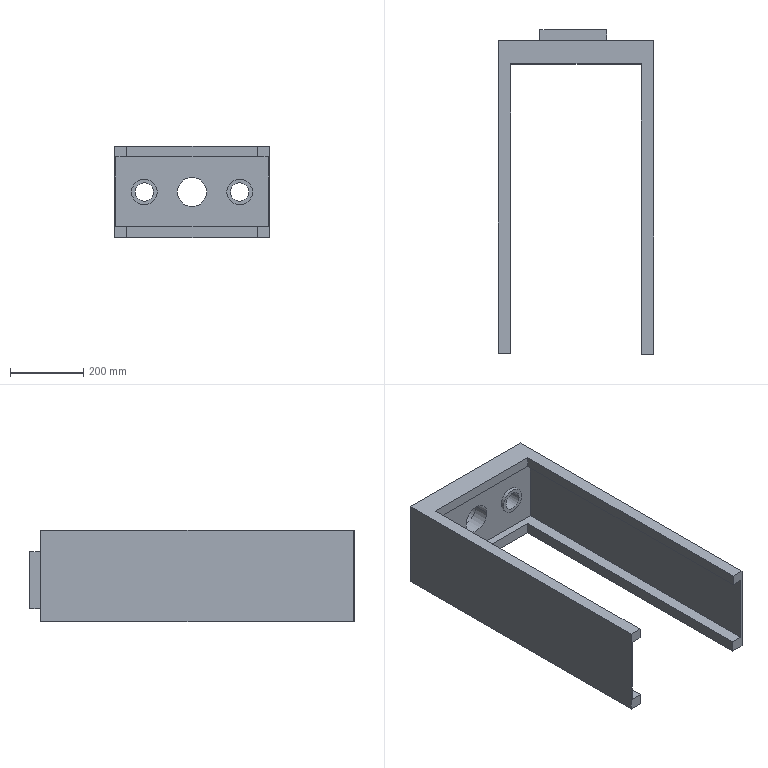Part | STEP file | Input 2 | 1 solid | 46 faces | box 425 x 886.727 x 250 mm | volume 9528731 mm3 | plane 32 | cylinder 14 | commonest cylinder face diameters 50 x4 70 x4 80 x2 85 x2 86 x2
STEP:
#1=CARTESIAN_POINT('',(-706.359,1977.264,3172.342));
#2=VERTEX_POINT('',#1);
#3=CARTESIAN_POINT('',(-791.359,1977.264,3172.342));
#4=VERTEX_POINT('',#3);
#5=CARTESIAN_POINT('',(-748.859,1977.264,3172.342));
#6=DIRECTION('',(0.,1.,0.));
#7=DIRECTION('',(1.,0.,0.));
#8=AXIS2_PLACEMENT_3D('',#5,#6,#7);
#9=CIRCLE('',#8,42.5);
#10=EDGE_CURVE('',#2,#4,#9,.T.);
#11=ORIENTED_EDGE('',*,*,#10,.F.);
#12=CARTESIAN_POINT('',(-706.359,1949.264,3172.342));
#13=VERTEX_POINT('',#12);
#14=CARTESIAN_POINT('',(-706.359,2599.264,3172.342));
#15=DIRECTION('',(0.,1.,0.));
#16=VECTOR('',#15,1000.);
#17=LINE('',#14,#16);
#18=EDGE_CURVE('',#13,#2,#17,.T.);
#19=ORIENTED_EDGE('',*,*,#18,.F.);
#20=CARTESIAN_POINT('',(-791.359,1949.264,3172.342));
#21=VERTEX_POINT('',#20);
#22=CARTESIAN_POINT('',(-748.859,1949.264,3172.342));
#23=DIRECTION('',(0.,1.,0.));
#24=DIRECTION('',(-1.,0.,0.));
#25=AXIS2_PLACEMENT_3D('',#22,#23,#24);
#26=CIRCLE('',#25,42.5);
#27=EDGE_CURVE('',#13,#21,#26,.T.);
#28=ORIENTED_EDGE('',*,*,#27,.T.);
#29=CARTESIAN_POINT('',(-791.359,2599.264,3172.342));
#30=DIRECTION('',(0.,1.,0.));
#31=VECTOR('',#30,1000.);
#32=LINE('',#29,#31);
#33=EDGE_CURVE('',#21,#4,#32,.T.);
#34=ORIENTED_EDGE('',*,*,#33,.T.);
#35=EDGE_LOOP('',(#11,#19,#28,#34));
#36=FACE_OUTER_BOUND('',#35,.T.);
#37=CARTESIAN_POINT('',(-748.859,2599.264,3172.342));
#38=DIRECTION('',(0.,-1.,0.));
#39=DIRECTION('',(1.,0.,0.));
#40=AXIS2_PLACEMENT_3D('',#37,#38,#39);
#41=CYLINDRICAL_SURFACE('',#40,42.5);
#42=ADVANCED_FACE('',(#36),#41,.T.);
#43=CARTESIAN_POINT('',(-791.859,1977.264,3172.342));
#44=VERTEX_POINT('',#43);
#45=CARTESIAN_POINT('',(-705.859,1977.264,3172.342));
#46=VERTEX_POINT('',#45);
#47=CARTESIAN_POINT('',(-748.859,1977.264,3172.342));
#48=DIRECTION('',(0.,1.,0.));
#49=DIRECTION('',(1.,0.,0.));
#50=AXIS2_PLACEMENT_3D('',#47,#48,#49);
#51=CIRCLE('',#50,43.);
#52=EDGE_CURVE('',#44,#46,#51,.T.);
#53=ORIENTED_EDGE('',*,*,#52,.F.);
#54=CARTESIAN_POINT('',(-791.859,1979.264,3172.342));
#55=VERTEX_POINT('',#54);
#56=CARTESIAN_POINT('',(-791.859,1977.264,3172.342));
#57=DIRECTION('',(0.,1.,0.));
#58=VECTOR('',#57,1000.);
#59=LINE('',#56,#58);
#60=EDGE_CURVE('',#44,#55,#59,.T.);
#61=ORIENTED_EDGE('',*,*,#60,.T.);
#62=CARTESIAN_POINT('',(-705.859,1979.264,3172.342));
#63=VERTEX_POINT('',#62);
#64=CARTESIAN_POINT('',(-748.859,1979.264,3172.342));
#65=DIRECTION('',(0.,1.,0.));
#66=DIRECTION('',(1.,0.,0.));
#67=AXIS2_PLACEMENT_3D('',#64,#65,#66);
#68=CIRCLE('',#67,43.);
#69=EDGE_CURVE('',#55,#63,#68,.T.);
#70=ORIENTED_EDGE('',*,*,#69,.T.);
#71=CARTESIAN_POINT('',(-705.859,1977.264,3172.342));
#72=DIRECTION('',(0.,1.,0.));
#73=VECTOR('',#72,1000.);
#74=LINE('',#71,#73);
#75=EDGE_CURVE('',#46,#63,#74,.T.);
#76=ORIENTED_EDGE('',*,*,#75,.F.);
#77=EDGE_LOOP('',(#53,#61,#70,#76));
#78=FACE_OUTER_BOUND('',#77,.T.);
#79=CARTESIAN_POINT('',(-748.859,1977.264,3172.342));
#80=DIRECTION('',(0.,1.,0.));
#81=DIRECTION('',(-1.,0.,0.));
#82=AXIS2_PLACEMENT_3D('',#79,#80,#81);
#83=CYLINDRICAL_SURFACE('',#82,43.);
#84=ADVANCED_FACE('',(#78),#83,.F.);
#85=CARTESIAN_POINT('',(-653.859,1895.264,3172.342));
#86=VERTEX_POINT('',#85);
#87=CARTESIAN_POINT('',(-583.859,1895.264,3172.342));
#88=VERTEX_POINT('',#87);
#89=CARTESIAN_POINT('',(-618.859,1895.264,3172.342));
#90=DIRECTION('',(0.,-1.,0.));
#91=DIRECTION('',(1.,0.,0.));
#92=AXIS2_PLACEMENT_3D('',#89,#90,#91);
#93=CIRCLE('',#92,35.);
#94=EDGE_CURVE('',#86,#88,#93,.T.);
#95=ORIENTED_EDGE('',*,*,#94,.F.);
#96=CARTESIAN_POINT('',(-653.859,1905.264,3172.342));
#97=VERTEX_POINT('',#96);
#98=CARTESIAN_POINT('',(-653.859,1895.264,3172.342));
#99=DIRECTION('',(0.,1.,0.));
#100=VECTOR('',#99,1000.);
#101=LINE('',#98,#100);
#102=EDGE_CURVE('',#86,#97,#101,.T.);
#103=ORIENTED_EDGE('',*,*,#102,.T.);
#104=CARTESIAN_POINT('',(-583.859,1905.264,3172.342));
#105=VERTEX_POINT('',#104);
#106=CARTESIAN_POINT('',(-618.859,1905.264,3172.342));
#107=DIRECTION('',(0.,-1.,0.));
#108=DIRECTION('',(1.,0.,0.));
#109=AXIS2_PLACEMENT_3D('',#106,#107,#108);
#110=CIRCLE('',#109,35.);
#111=EDGE_CURVE('',#97,#105,#110,.T.);
#112=ORIENTED_EDGE('',*,*,#111,.T.);
#113=CARTESIAN_POINT('',(-583.859,1895.264,3172.342));
#114=DIRECTION('',(0.,1.,0.));
#115=VECTOR('',#114,1000.);
#116=LINE('',#113,#115);
#117=EDGE_CURVE('',#88,#105,#116,.T.);
#118=ORIENTED_EDGE('',*,*,#117,.F.);
#119=EDGE_LOOP('',(#95,#103,#112,#118));
#120=FACE_OUTER_BOUND('',#119,.T.);
#121=CARTESIAN_POINT('',(-618.859,1895.264,3172.342));
#122=DIRECTION('',(0.,1.,0.));
#123=DIRECTION('',(-1.,0.,0.));
#124=AXIS2_PLACEMENT_3D('',#121,#122,#123);
#125=CYLINDRICAL_SURFACE('',#124,35.);
#126=ADVANCED_FACE('',(#120),#125,.T.);
#127=CARTESIAN_POINT('',(-913.859,1895.264,3172.342));
#128=VERTEX_POINT('',#127);
#129=CARTESIAN_POINT('',(-843.859,1895.264,3172.342));
#130=VERTEX_POINT('',#129);
#131=CARTESIAN_POINT('',(-878.859,1895.264,3172.342));
#132=DIRECTION('',(0.,-1.,0.));
#133=DIRECTION('',(-1.,0.,0.));
#134=AXIS2_PLACEMENT_3D('',#131,#132,#133);
#135=CIRCLE('',#134,35.);
#136=EDGE_CURVE('',#128,#130,#135,.T.);
#137=ORIENTED_EDGE('',*,*,#136,.F.);
#138=CARTESIAN_POINT('',(-913.859,1905.264,3172.342));
#139=VERTEX_POINT('',#138);
#140=CARTESIAN_POINT('',(-913.859,1895.264,3172.342));
#141=DIRECTION('',(0.,1.,0.));
#142=VECTOR('',#141,1000.);
#143=LINE('',#140,#142);
#144=EDGE_CURVE('',#128,#139,#143,.T.);
#145=ORIENTED_EDGE('',*,*,#144,.T.);
#146=CARTESIAN_POINT('',(-843.859,1905.264,3172.342));
#147=VERTEX_POINT('',#146);
#148=CARTESIAN_POINT('',(-878.859,1905.264,3172.342));
#149=DIRECTION('',(0.,-1.,0.));
#150=DIRECTION('',(1.,0.,0.));
#151=AXIS2_PLACEMENT_3D('',#148,#149,#150);
#152=CIRCLE('',#151,35.);
#153=EDGE_CURVE('',#139,#147,#152,.T.);
#154=ORIENTED_EDGE('',*,*,#153,.T.);
#155=CARTESIAN_POINT('',(-843.859,1895.264,3172.342));
#156=DIRECTION('',(0.,1.,0.));
#157=VECTOR('',#156,1000.);
#158=LINE('',#155,#157);
#159=EDGE_CURVE('',#130,#147,#158,.T.);
#160=ORIENTED_EDGE('',*,*,#159,.F.);
#161=EDGE_LOOP('',(#137,#145,#154,#160));
#162=FACE_OUTER_BOUND('',#161,.T.);
#163=CARTESIAN_POINT('',(-878.859,1895.264,3172.342));
#164=DIRECTION('',(0.,1.,0.));
#165=DIRECTION('',(-1.,0.,0.));
#166=AXIS2_PLACEMENT_3D('',#163,#164,#165);
#167=CYLINDRICAL_SURFACE('',#166,35.);
#168=ADVANCED_FACE('',(#162),#167,.T.);
#169=CARTESIAN_POINT('',(-853.859,1949.264,3172.342));
#170=VERTEX_POINT('',#169);
#171=CARTESIAN_POINT('',(-903.859,1949.264,3172.342));
#172=VERTEX_POINT('',#171);
#173=CARTESIAN_POINT('',(-878.859,1949.264,3172.342));
#174=DIRECTION('',(0.,-1.,0.));
#175=DIRECTION('',(-1.,0.,0.));
#176=AXIS2_PLACEMENT_3D('',#173,#174,#175);
#177=CIRCLE('',#176,25.);
#178=EDGE_CURVE('',#170,#172,#177,.T.);
#179=ORIENTED_EDGE('',*,*,#178,.F.);
#180=CARTESIAN_POINT('',(-853.859,1895.264,3172.342));
#181=VERTEX_POINT('',#180);
#182=CARTESIAN_POINT('',(-853.859,2789.264,3172.342));
#183=DIRECTION('',(0.,1.,0.));
#184=VECTOR('',#183,1000.);
#185=LINE('',#182,#184);
#186=EDGE_CURVE('',#181,#170,#185,.T.);
#187=ORIENTED_EDGE('',*,*,#186,.F.);
#188=CARTESIAN_POINT('',(-903.859,1895.264,3172.342));
#189=VERTEX_POINT('',#188);
#190=CARTESIAN_POINT('',(-878.859,1895.264,3172.342));
#191=DIRECTION('',(0.,-1.,0.));
#192=DIRECTION('',(-1.,0.,0.));
#193=AXIS2_PLACEMENT_3D('',#190,#191,#192);
#194=CIRCLE('',#193,25.);
#195=EDGE_CURVE('',#181,#189,#194,.T.);
#196=ORIENTED_EDGE('',*,*,#195,.T.);
#197=CARTESIAN_POINT('',(-903.859,2789.264,3172.342));
#198=DIRECTION('',(0.,1.,0.));
#199=VECTOR('',#198,1000.);
#200=LINE('',#197,#199);
#201=EDGE_CURVE('',#189,#172,#200,.T.);
#202=ORIENTED_EDGE('',*,*,#201,.T.);
#203=EDGE_LOOP('',(#179,#187,#196,#202));
#204=FACE_OUTER_BOUND('',#203,.T.);
#205=CARTESIAN_POINT('',(-878.859,2789.264,3172.342));
#206=DIRECTION('',(0.,-1.,0.));
#207=DIRECTION('',(1.,0.,0.));
#208=AXIS2_PLACEMENT_3D('',#205,#206,#207);
#209=CYLINDRICAL_SURFACE('',#208,25.);
#210=ADVANCED_FACE('',(#204),#209,.F.);
#211=CARTESIAN_POINT('',(-593.859,1949.264,3172.342));
#212=VERTEX_POINT('',#211);
#213=CARTESIAN_POINT('',(-643.859,1949.264,3172.342));
#214=VERTEX_POINT('',#213);
#215=CARTESIAN_POINT('',(-618.859,1949.264,3172.342));
#216=DIRECTION('',(0.,-1.,0.));
#217=DIRECTION('',(-1.,0.,0.));
#218=AXIS2_PLACEMENT_3D('',#215,#216,#217);
#219=CIRCLE('',#218,25.);
#220=EDGE_CURVE('',#212,#214,#219,.T.);
#221=ORIENTED_EDGE('',*,*,#220,.F.);
#222=CARTESIAN_POINT('',(-593.859,1895.264,3172.342));
#223=VERTEX_POINT('',#222);
#224=CARTESIAN_POINT('',(-593.859,2789.264,3172.342));
#225=DIRECTION('',(0.,1.,0.));
#226=VECTOR('',#225,1000.);
#227=LINE('',#224,#226);
#228=EDGE_CURVE('',#223,#212,#227,.T.);
#229=ORIENTED_EDGE('',*,*,#228,.F.);
#230=CARTESIAN_POINT('',(-643.859,1895.264,3172.342));
#231=VERTEX_POINT('',#230);
#232=CARTESIAN_POINT('',(-618.859,1895.264,3172.342));
#233=DIRECTION('',(0.,-1.,0.));
#234=DIRECTION('',(-1.,0.,0.));
#235=AXIS2_PLACEMENT_3D('',#232,#233,#234);
#236=CIRCLE('',#235,25.);
#237=EDGE_CURVE('',#223,#231,#236,.T.);
#238=ORIENTED_EDGE('',*,*,#237,.T.);
#239=CARTESIAN_POINT('',(-643.859,2789.264,3172.342));
#240=DIRECTION('',(0.,1.,0.));
#241=VECTOR('',#240,1000.);
#242=LINE('',#239,#241);
#243=EDGE_CURVE('',#231,#214,#242,.T.);
#244=ORIENTED_EDGE('',*,*,#243,.T.);
#245=EDGE_LOOP('',(#221,#229,#238,#244));
#246=FACE_OUTER_BOUND('',#245,.T.);
#247=CARTESIAN_POINT('',(-618.859,2789.264,3172.342));
#248=DIRECTION('',(0.,-1.,0.));
#249=DIRECTION('',(1.,0.,0.));
#250=AXIS2_PLACEMENT_3D('',#247,#248,#249);
#251=CYLINDRICAL_SURFACE('',#250,25.);
#252=ADVANCED_FACE('',(#246),#251,.F.);
#253=CARTESIAN_POINT('',(-708.859,1977.264,3172.342));
#254=VERTEX_POINT('',#253);
#255=CARTESIAN_POINT('',(-788.859,1977.264,3172.342));
#256=VERTEX_POINT('',#255);
#257=CARTESIAN_POINT('',(-748.859,1977.264,3172.342));
#258=DIRECTION('',(0.,-1.,0.));
#259=DIRECTION('',(1.,0.,0.));
#260=AXIS2_PLACEMENT_3D('',#257,#258,#259);
#261=CIRCLE('',#260,40.);
#262=EDGE_CURVE('',#254,#256,#261,.T.);
#263=ORIENTED_EDGE('',*,*,#262,.F.);
#264=CARTESIAN_POINT('',(-708.859,1905.264,3172.342));
#265=VERTEX_POINT('',#264);
#266=CARTESIAN_POINT('',(-708.859,2829.064,3172.342));
#267=DIRECTION('',(0.,1.,0.));
#268=VECTOR('',#267,1000.);
#269=LINE('',#266,#268);
#270=EDGE_CURVE('',#265,#254,#269,.T.);
#271=ORIENTED_EDGE('',*,*,#270,.F.);
#272=CARTESIAN_POINT('',(-788.859,1905.264,3172.342));
#273=VERTEX_POINT('',#272);
#274=CARTESIAN_POINT('',(-748.859,1905.264,3172.342));
#275=DIRECTION('',(0.,1.,0.));
#276=DIRECTION('',(1.,0.,0.));
#277=AXIS2_PLACEMENT_3D('',#274,#275,#276);
#278=CIRCLE('',#277,40.);
#279=EDGE_CURVE('',#273,#265,#278,.T.);
#280=ORIENTED_EDGE('',*,*,#279,.F.);
#281=CARTESIAN_POINT('',(-788.859,2829.064,3172.342));
#282=DIRECTION('',(0.,1.,0.));
#283=VECTOR('',#282,1000.);
#284=LINE('',#281,#283);
#285=EDGE_CURVE('',#273,#256,#284,.T.);
#286=ORIENTED_EDGE('',*,*,#285,.T.);
#287=EDGE_LOOP('',(#263,#271,#280,#286));
#288=FACE_OUTER_BOUND('',#287,.T.);
#289=CARTESIAN_POINT('',(-748.859,2829.064,3172.342));
#290=DIRECTION('',(0.,-1.,0.));
#291=DIRECTION('',(1.,0.,0.));
#292=AXIS2_PLACEMENT_3D('',#289,#290,#291);
#293=CYLINDRICAL_SURFACE('',#292,40.);
#294=ADVANCED_FACE('',(#288),#293,.F.);
#295=CARTESIAN_POINT('',(-961.359,1949.264,3047.342));
#296=VERTEX_POINT('',#295);
#297=CARTESIAN_POINT('',(-961.359,1095.094,3047.342));
#298=VERTEX_POINT('',#297);
#299=CARTESIAN_POINT('',(-961.359,1949.264,3047.342));
#300=DIRECTION('',(0.,-1.,0.));
#301=VECTOR('',#300,1000.);
#302=LINE('',#299,#301);
#303=EDGE_CURVE('',#296,#298,#302,.T.);
#304=ORIENTED_EDGE('',*,*,#303,.T.);
#305=CARTESIAN_POINT('',(-961.359,1095.094,3297.342));
#306=VERTEX_POINT('',#305);
#307=CARTESIAN_POINT('',(-961.359,1095.094,4799.342));
#308=DIRECTION('',(0.,0.,-1.));
#309=VECTOR('',#308,1000.);
#310=LINE('',#307,#309);
#311=EDGE_CURVE('',#306,#298,#310,.T.);
#312=ORIENTED_EDGE('',*,*,#311,.F.);
#313=CARTESIAN_POINT('',(-961.359,1949.264,3297.342));
#314=VERTEX_POINT('',#313);
#315=CARTESIAN_POINT('',(-961.359,1949.264,3297.342));
#316=DIRECTION('',(0.,-1.,0.));
#317=VECTOR('',#316,1000.);
#318=LINE('',#315,#317);
#319=EDGE_CURVE('',#314,#306,#318,.T.);
#320=ORIENTED_EDGE('',*,*,#319,.F.);
#321=CARTESIAN_POINT('',(-961.359,1949.264,3297.342));
#322=DIRECTION('',(0.,0.,1.));
#323=VECTOR('',#322,1000.);
#324=LINE('',#321,#323);
#325=EDGE_CURVE('',#296,#314,#324,.T.);
#326=ORIENTED_EDGE('',*,*,#325,.F.);
#327=EDGE_LOOP('',(#304,#312,#320,#326));
#328=FACE_OUTER_BOUND('',#327,.T.);
#329=CARTESIAN_POINT('',(-961.359,1949.264,3297.342));
#330=DIRECTION('',(1.,0.,0.));
#331=DIRECTION('',(0.,1.,0.));
#332=AXIS2_PLACEMENT_3D('',#329,#330,#331);
#333=PLANE('',#332);
#334=ADVANCED_FACE('',(#328),#333,.F.);
#335=CARTESIAN_POINT('',(-536.359,1949.264,3297.342));
#336=VERTEX_POINT('',#335);
#337=CARTESIAN_POINT('',(-536.359,1092.538,3297.342));
#338=VERTEX_POINT('',#337);
#339=CARTESIAN_POINT('',(-536.359,1949.264,3297.342));
#340=DIRECTION('',(0.,-1.,0.));
#341=VECTOR('',#340,1000.);
#342=LINE('',#339,#341);
#343=EDGE_CURVE('',#336,#338,#342,.T.);
#344=ORIENTED_EDGE('',*,*,#343,.T.);
#345=CARTESIAN_POINT('',(-536.359,1092.538,3047.342));
#346=VERTEX_POINT('',#345);
#347=CARTESIAN_POINT('',(-536.359,1092.538,4799.342));
#348=DIRECTION('',(0.,0.,-1.));
#349=VECTOR('',#348,1000.);
#350=LINE('',#347,#349);
#351=EDGE_CURVE('',#338,#346,#350,.T.);
#352=ORIENTED_EDGE('',*,*,#351,.T.);
#353=CARTESIAN_POINT('',(-536.359,1949.264,3047.342));
#354=VERTEX_POINT('',#353);
#355=CARTESIAN_POINT('',(-536.359,1949.264,3047.342));
#356=DIRECTION('',(0.,-1.,0.));
#357=VECTOR('',#356,1000.);
#358=LINE('',#355,#357);
#359=EDGE_CURVE('',#354,#346,#358,.T.);
#360=ORIENTED_EDGE('',*,*,#359,.F.);
#361=CARTESIAN_POINT('',(-536.359,1949.264,3297.342));
#362=DIRECTION('',(0.,0.,-1.));
#363=VECTOR('',#362,1000.);
#364=LINE('',#361,#363);
#365=EDGE_CURVE('',#336,#354,#364,.T.);
#366=ORIENTED_EDGE('',*,*,#365,.F.);
#367=EDGE_LOOP('',(#344,#352,#360,#366));
#368=FACE_OUTER_BOUND('',#367,.T.);
#369=CARTESIAN_POINT('',(-536.359,1949.264,3297.342));
#370=DIRECTION('',(-1.,0.,0.));
#371=DIRECTION('',(0.,-1.,0.));
#372=AXIS2_PLACEMENT_3D('',#369,#370,#371);
#373=PLANE('',#372);
#374=ADVANCED_FACE('',(#368),#373,.F.);
#375=ORIENTED_EDGE('',*,*,#359,.T.);
#376=CARTESIAN_POINT('',(-571.359,1092.538,3047.342));
#377=VERTEX_POINT('',#376);
#378=CARTESIAN_POINT('',(-683.964,1092.538,3047.342));
#379=DIRECTION('',(1.,0.,0.));
#380=VECTOR('',#379,1000.);
#381=LINE('',#378,#380);
#382=EDGE_CURVE('',#377,#346,#381,.T.);
#383=ORIENTED_EDGE('',*,*,#382,.F.);
#384=CARTESIAN_POINT('',(-571.359,1884.264,3047.342));
#385=VERTEX_POINT('',#384);
#386=CARTESIAN_POINT('',(-571.359,890.264,3047.342));
#387=DIRECTION('',(0.,-1.,0.));
#388=VECTOR('',#387,1000.);
#389=LINE('',#386,#388);
#390=EDGE_CURVE('',#385,#377,#389,.T.);
#391=ORIENTED_EDGE('',*,*,#390,.F.);
#392=CARTESIAN_POINT('',(-926.359,1884.264,3047.342));
#393=VERTEX_POINT('',#392);
#394=CARTESIAN_POINT('',(-926.359,1884.264,3047.342));
#395=DIRECTION('',(1.,0.,0.));
#396=VECTOR('',#395,1000.);
#397=LINE('',#394,#396);
#398=EDGE_CURVE('',#393,#385,#397,.T.);
#399=ORIENTED_EDGE('',*,*,#398,.F.);
#400=CARTESIAN_POINT('',(-926.359,1095.094,3047.342));
#401=VERTEX_POINT('',#400);
#402=CARTESIAN_POINT('',(-926.359,890.264,3047.342));
#403=DIRECTION('',(0.,1.,0.));
#404=VECTOR('',#403,1000.);
#405=LINE('',#402,#404);
#406=EDGE_CURVE('',#401,#393,#405,.T.);
#407=ORIENTED_EDGE('',*,*,#406,.F.);
#408=CARTESIAN_POINT('',(-819.635,1095.094,3047.342));
#409=DIRECTION('',(1.,0.,0.));
#410=VECTOR('',#409,1000.);
#411=LINE('',#408,#410);
#412=EDGE_CURVE('',#298,#401,#411,.T.);
#413=ORIENTED_EDGE('',*,*,#412,.F.);
#414=ORIENTED_EDGE('',*,*,#303,.F.);
#415=CARTESIAN_POINT('',(-961.359,1949.264,3047.342));
#416=DIRECTION('',(-1.,0.,0.));
#417=VECTOR('',#416,1000.);
#418=LINE('',#415,#417);
#419=EDGE_CURVE('',#354,#296,#418,.T.);
#420=ORIENTED_EDGE('',*,*,#419,.F.);
#421=EDGE_LOOP('',(#375,#383,#391,#399,#407,#413,#414,#420));
#422=FACE_OUTER_BOUND('',#421,.T.);
#423=CARTESIAN_POINT('',(-961.359,1949.264,3047.342));
#424=DIRECTION('',(0.,0.,1.));
#425=DIRECTION('',(0.,1.,0.));
#426=AXIS2_PLACEMENT_3D('',#423,#424,#425);
#427=PLANE('',#426);
#428=ADVANCED_FACE('',(#422),#427,.F.);
#429=CARTESIAN_POINT('',(-570.359,1885.264,3297.342));
#430=VERTEX_POINT('',#429);
#431=CARTESIAN_POINT('',(-570.359,1092.538,3297.342));
#432=VERTEX_POINT('',#431);
#433=CARTESIAN_POINT('',(-570.359,1949.264,3297.342));
#434=DIRECTION('',(0.,-1.,0.));
#435=VECTOR('',#434,1000.);
#436=LINE('',#433,#435);
#437=EDGE_CURVE('',#430,#432,#436,.T.);
#438=ORIENTED_EDGE('',*,*,#437,.T.);
#439=CARTESIAN_POINT('',(-961.359,1092.538,3297.342));
#440=DIRECTION('',(1.,0.,0.));
#441=VECTOR('',#440,1000.);
#442=LINE('',#439,#441);
#443=EDGE_CURVE('',#432,#338,#442,.T.);
#444=ORIENTED_EDGE('',*,*,#443,.T.);
#445=ORIENTED_EDGE('',*,*,#343,.F.);
#446=CARTESIAN_POINT('',(-961.359,1949.264,3297.342));
#447=DIRECTION('',(1.,0.,0.));
#448=VECTOR('',#447,1000.);
#449=LINE('',#446,#448);
#450=EDGE_CURVE('',#314,#336,#449,.T.);
#451=ORIENTED_EDGE('',*,*,#450,.F.);
#452=ORIENTED_EDGE('',*,*,#319,.T.);
#453=CARTESIAN_POINT('',(-927.359,1095.094,3297.342));
#454=VERTEX_POINT('',#453);
#455=CARTESIAN_POINT('',(-961.359,1095.094,3297.342));
#456=DIRECTION('',(1.,0.,0.));
#457=VECTOR('',#456,1000.);
#458=LINE('',#455,#457);
#459=EDGE_CURVE('',#306,#454,#458,.T.);
#460=ORIENTED_EDGE('',*,*,#459,.T.);
#461=CARTESIAN_POINT('',(-927.359,1885.264,3297.342));
#462=VERTEX_POINT('',#461);
#463=CARTESIAN_POINT('',(-927.359,1949.264,3297.342));
#464=DIRECTION('',(0.,1.,0.));
#465=VECTOR('',#464,1000.);
#466=LINE('',#463,#465);
#467=EDGE_CURVE('',#454,#462,#466,.T.);
#468=ORIENTED_EDGE('',*,*,#467,.T.);
#469=CARTESIAN_POINT('',(-961.359,1885.264,3297.342));
#470=DIRECTION('',(1.,0.,0.));
#471=VECTOR('',#470,1000.);
#472=LINE('',#469,#471);
#473=EDGE_CURVE('',#462,#430,#472,.T.);
#474=ORIENTED_EDGE('',*,*,#473,.T.);
#475=EDGE_LOOP('',(#438,#444,#445,#451,#452,#460,#468,#474));
#476=FACE_OUTER_BOUND('',#475,.T.);
#477=CARTESIAN_POINT('',(-961.359,1949.264,3297.342));
#478=DIRECTION('',(0.,0.,-1.));
#479=DIRECTION('',(0.,-1.,0.));
#480=AXIS2_PLACEMENT_3D('',#477,#478,#479);
#481=PLANE('',#480);
#482=ADVANCED_FACE('',(#476),#481,.F.);
#483=CARTESIAN_POINT('',(-571.359,1884.264,3078.342));
#484=VERTEX_POINT('',#483);
#485=CARTESIAN_POINT('',(-571.359,1092.538,3078.342));
#486=VERTEX_POINT('',#485);
#487=CARTESIAN_POINT('',(-571.359,890.264,3078.342));
#488=DIRECTION('',(0.,-1.,0.));
#489=VECTOR('',#488,1000.);
#490=LINE('',#487,#489);
#491=EDGE_CURVE('',#484,#486,#490,.T.);
#492=ORIENTED_EDGE('',*,*,#491,.T.);
#493=CARTESIAN_POINT('',(-540.359,1092.538,3078.342));
#494=VERTEX_POINT('',#493);
#495=CARTESIAN_POINT('',(-748.859,1092.538,3078.342));
#496=DIRECTION('',(1.,0.,0.));
#497=VECTOR('',#496,1000.);
#498=LINE('',#495,#497);
#499=EDGE_CURVE('',#486,#494,#498,.T.);
#500=ORIENTED_EDGE('',*,*,#499,.T.);
#501=CARTESIAN_POINT('',(-540.359,1905.264,3078.342));
#502=VERTEX_POINT('',#501);
#503=CARTESIAN_POINT('',(-540.359,869.264,3078.342));
#504=DIRECTION('',(0.,-1.,0.));
#505=VECTOR('',#504,1000.);
#506=LINE('',#503,#505);
#507=EDGE_CURVE('',#502,#494,#506,.T.);
#508=ORIENTED_EDGE('',*,*,#507,.F.);
#509=CARTESIAN_POINT('',(-957.359,1905.264,3078.342));
#510=VERTEX_POINT('',#509);
#511=CARTESIAN_POINT('',(-957.359,1905.264,3078.342));
#512=DIRECTION('',(1.,0.,0.));
#513=VECTOR('',#512,1000.);
#514=LINE('',#511,#513);
#515=EDGE_CURVE('',#510,#502,#514,.T.);
#516=ORIENTED_EDGE('',*,*,#515,.F.);
#517=CARTESIAN_POINT('',(-957.359,1095.094,3078.342));
#518=VERTEX_POINT('',#517);
#519=CARTESIAN_POINT('',(-957.359,869.264,3078.342));
#520=DIRECTION('',(0.,1.,0.));
#521=VECTOR('',#520,1000.);
#522=LINE('',#519,#521);
#523=EDGE_CURVE('',#518,#510,#522,.T.);
#524=ORIENTED_EDGE('',*,*,#523,.F.);
#525=CARTESIAN_POINT('',(-926.359,1095.094,3078.342));
#526=VERTEX_POINT('',#525);
#527=CARTESIAN_POINT('',(-748.859,1095.094,3078.342));
#528=DIRECTION('',(1.,0.,0.));
#529=VECTOR('',#528,1000.);
#530=LINE('',#527,#529);
#531=EDGE_CURVE('',#518,#526,#530,.T.);
#532=ORIENTED_EDGE('',*,*,#531,.T.);
#533=CARTESIAN_POINT('',(-926.359,1884.264,3078.342));
#534=VERTEX_POINT('',#533);
#535=CARTESIAN_POINT('',(-926.359,890.264,3078.342));
#536=DIRECTION('',(0.,1.,0.));
#537=VECTOR('',#536,1000.);
#538=LINE('',#535,#537);
#539=EDGE_CURVE('',#526,#534,#538,.T.);
#540=ORIENTED_EDGE('',*,*,#539,.T.);
#541=CARTESIAN_POINT('',(-926.359,1884.264,3078.342));
#542=DIRECTION('',(1.,0.,0.));
#543=VECTOR('',#542,1000.);
#544=LINE('',#541,#543);
#545=EDGE_CURVE('',#534,#484,#544,.T.);
#546=ORIENTED_EDGE('',*,*,#545,.T.);
#547=EDGE_LOOP('',(#492,#500,#508,#516,#524,#532,#540,#546));
#548=FACE_OUTER_BOUND('',#547,.T.);
#549=CARTESIAN_POINT('',(-748.859,825.264,3078.342));
#550=DIRECTION('',(0.,0.,-1.));
#551=DIRECTION('',(0.,-1.,0.));
#552=AXIS2_PLACEMENT_3D('',#549,#550,#551);
#553=PLANE('',#552);
#554=ADVANCED_FACE('',(#548),#553,.F.);
#555=CARTESIAN_POINT('',(-957.359,1095.094,3268.342));
#556=VERTEX_POINT('',#555);
#557=CARTESIAN_POINT('',(-957.359,1905.264,3268.342));
#558=VERTEX_POINT('',#557);
#559=CARTESIAN_POINT('',(-957.359,869.264,3268.342));
#560=DIRECTION('',(0.,1.,0.));
#561=VECTOR('',#560,1000.);
#562=LINE('',#559,#561);
#563=EDGE_CURVE('',#556,#558,#562,.T.);
#564=ORIENTED_EDGE('',*,*,#563,.F.);
#565=CARTESIAN_POINT('',(-957.359,1095.094,3268.342));
#566=DIRECTION('',(0.,0.,-1.));
#567=VECTOR('',#566,1000.);
#568=LINE('',#565,#567);
#569=EDGE_CURVE('',#556,#518,#568,.T.);
#570=ORIENTED_EDGE('',*,*,#569,.T.);
#571=ORIENTED_EDGE('',*,*,#523,.T.);
#572=CARTESIAN_POINT('',(-957.359,1905.264,3268.342));
#573=DIRECTION('',(0.,0.,-1.));
#574=VECTOR('',#573,1000.);
#575=LINE('',#572,#574);
#576=EDGE_CURVE('',#558,#510,#575,.T.);
#577=ORIENTED_EDGE('',*,*,#576,.F.);
#578=EDGE_LOOP('',(#564,#570,#571,#577));
#579=FACE_OUTER_BOUND('',#578,.T.);
#580=CARTESIAN_POINT('',(-957.359,869.264,3268.342));
#581=DIRECTION('',(-1.,0.,0.));
#582=DIRECTION('',(0.,-1.,0.));
#583=AXIS2_PLACEMENT_3D('',#580,#581,#582);
#584=PLANE('',#583);
#585=ADVANCED_FACE('',(#579),#584,.F.);
#586=ORIENTED_EDGE('',*,*,#507,.T.);
#587=CARTESIAN_POINT('',(-540.359,1092.538,3268.342));
#588=VERTEX_POINT('',#587);
#589=CARTESIAN_POINT('',(-540.359,1092.538,3268.342));
#590=DIRECTION('',(0.,0.,1.));
#591=VECTOR('',#590,1000.);
#592=LINE('',#589,#591);
#593=EDGE_CURVE('',#494,#588,#592,.T.);
#594=ORIENTED_EDGE('',*,*,#593,.T.);
#595=CARTESIAN_POINT('',(-540.359,1905.264,3268.342));
#596=VERTEX_POINT('',#595);
#597=CARTESIAN_POINT('',(-540.359,869.264,3268.342));
#598=DIRECTION('',(0.,-1.,0.));
#599=VECTOR('',#598,1000.);
#600=LINE('',#597,#599);
#601=EDGE_CURVE('',#596,#588,#600,.T.);
#602=ORIENTED_EDGE('',*,*,#601,.F.);
#603=CARTESIAN_POINT('',(-540.359,1905.264,3268.342));
#604=DIRECTION('',(0.,0.,-1.));
#605=VECTOR('',#604,1000.);
#606=LINE('',#603,#605);
#607=EDGE_CURVE('',#596,#502,#606,.T.);
#608=ORIENTED_EDGE('',*,*,#607,.T.);
#609=EDGE_LOOP('',(#586,#594,#602,#608));
#610=FACE_OUTER_BOUND('',#609,.T.);
#611=CARTESIAN_POINT('',(-540.359,869.264,3268.342));
#612=DIRECTION('',(1.,0.,0.));
#613=DIRECTION('',(0.,1.,0.));
#614=AXIS2_PLACEMENT_3D('',#611,#612,#613);
#615=PLANE('',#614);
#616=ADVANCED_FACE('',(#610),#615,.F.);
#617=CARTESIAN_POINT('',(-570.359,1092.538,3268.342));
#618=VERTEX_POINT('',#617);
#619=CARTESIAN_POINT('',(-748.859,1092.538,3268.342));
#620=DIRECTION('',(1.,0.,0.));
#621=VECTOR('',#620,1000.);
#622=LINE('',#619,#621);
#623=EDGE_CURVE('',#618,#588,#622,.T.);
#624=ORIENTED_EDGE('',*,*,#623,.F.);
#625=CARTESIAN_POINT('',(-570.359,1885.264,3268.342));
#626=VERTEX_POINT('',#625);
#627=CARTESIAN_POINT('',(-570.359,889.264,3268.342));
#628=DIRECTION('',(0.,-1.,0.));
#629=VECTOR('',#628,1000.);
#630=LINE('',#627,#629);
#631=EDGE_CURVE('',#626,#618,#630,.T.);
#632=ORIENTED_EDGE('',*,*,#631,.F.);
#633=CARTESIAN_POINT('',(-927.359,1885.264,3268.342));
#634=VERTEX_POINT('',#633);
#635=CARTESIAN_POINT('',(-927.359,1885.264,3268.342));
#636=DIRECTION('',(1.,0.,0.));
#637=VECTOR('',#636,1000.);
#638=LINE('',#635,#637);
#639=EDGE_CURVE('',#634,#626,#638,.T.);
#640=ORIENTED_EDGE('',*,*,#639,.F.);
#641=CARTESIAN_POINT('',(-927.359,1095.094,3268.342));
#642=VERTEX_POINT('',#641);
#643=CARTESIAN_POINT('',(-927.359,889.264,3268.342));
#644=DIRECTION('',(0.,1.,0.));
#645=VECTOR('',#644,1000.);
#646=LINE('',#643,#645);
#647=EDGE_CURVE('',#642,#634,#646,.T.);
#648=ORIENTED_EDGE('',*,*,#647,.F.);
#649=CARTESIAN_POINT('',(-748.859,1095.094,3268.342));
#650=DIRECTION('',(1.,0.,0.));
#651=VECTOR('',#650,1000.);
#652=LINE('',#649,#651);
#653=EDGE_CURVE('',#556,#642,#652,.T.);
#654=ORIENTED_EDGE('',*,*,#653,.F.);
#655=ORIENTED_EDGE('',*,*,#563,.T.);
#656=CARTESIAN_POINT('',(-957.359,1905.264,3268.342));
#657=DIRECTION('',(1.,0.,0.));
#658=VECTOR('',#657,1000.);
#659=LINE('',#656,#658);
#660=EDGE_CURVE('',#558,#596,#659,.T.);
#661=ORIENTED_EDGE('',*,*,#660,.T.);
#662=ORIENTED_EDGE('',*,*,#601,.T.);
#663=EDGE_LOOP('',(#624,#632,#640,#648,#654,#655,#661,#662));
#664=FACE_OUTER_BOUND('',#663,.T.);
#665=CARTESIAN_POINT('',(-748.859,825.264,3268.342));
#666=DIRECTION('',(0.,0.,-1.));
#667=DIRECTION('',(0.,-1.,0.));
#668=AXIS2_PLACEMENT_3D('',#665,#666,#667);
#669=PLANE('',#668);
#670=ADVANCED_FACE('',(#664),#669,.T.);
#671=ORIENTED_EDGE('',*,*,#631,.T.);
#672=CARTESIAN_POINT('',(-570.359,1092.538,3458.342));
#673=DIRECTION('',(0.,0.,1.));
#674=VECTOR('',#673,1000.);
#675=LINE('',#672,#674);
#676=EDGE_CURVE('',#618,#432,#675,.T.);
#677=ORIENTED_EDGE('',*,*,#676,.T.);
#678=ORIENTED_EDGE('',*,*,#437,.F.);
#679=CARTESIAN_POINT('',(-570.359,1885.264,3458.342));
#680=DIRECTION('',(0.,0.,-1.));
#681=VECTOR('',#680,1000.);
#682=LINE('',#679,#681);
#683=EDGE_CURVE('',#430,#626,#682,.T.);
#684=ORIENTED_EDGE('',*,*,#683,.T.);
#685=EDGE_LOOP('',(#671,#677,#678,#684));
#686=FACE_OUTER_BOUND('',#685,.T.);
#687=CARTESIAN_POINT('',(-570.359,889.264,3458.342));
#688=DIRECTION('',(1.,0.,0.));
#689=DIRECTION('',(0.,1.,0.));
#690=AXIS2_PLACEMENT_3D('',#687,#688,#689);
#691=PLANE('',#690);
#692=ADVANCED_FACE('',(#686),#691,.F.);
#693=ORIENTED_EDGE('',*,*,#467,.F.);
#694=CARTESIAN_POINT('',(-927.359,1095.094,3458.342));
#695=DIRECTION('',(0.,0.,-1.));
#696=VECTOR('',#695,1000.);
#697=LINE('',#694,#696);
#698=EDGE_CURVE('',#454,#642,#697,.T.);
#699=ORIENTED_EDGE('',*,*,#698,.T.);
#700=ORIENTED_EDGE('',*,*,#647,.T.);
#701=CARTESIAN_POINT('',(-927.359,1885.264,3458.342));
#702=DIRECTION('',(0.,0.,-1.));
#703=VECTOR('',#702,1000.);
#704=LINE('',#701,#703);
#705=EDGE_CURVE('',#462,#634,#704,.T.);
#706=ORIENTED_EDGE('',*,*,#705,.F.);
#707=EDGE_LOOP('',(#693,#699,#700,#706));
#708=FACE_OUTER_BOUND('',#707,.T.);
#709=CARTESIAN_POINT('',(-927.359,889.264,3458.342));
#710=DIRECTION('',(-1.,0.,0.));
#711=DIRECTION('',(0.,-1.,0.));
#712=AXIS2_PLACEMENT_3D('',#709,#710,#711);
#713=PLANE('',#712);
#714=ADVANCED_FACE('',(#708),#713,.F.);
#715=CARTESIAN_POINT('',(-748.859,1979.264,3172.342));
#716=DIRECTION('',(0.,1.,0.));
#717=DIRECTION('',(1.,0.,0.));
#718=AXIS2_PLACEMENT_3D('',#715,#716,#717);
#719=CIRCLE('',#718,43.);
#720=EDGE_CURVE('',#63,#55,#719,.T.);
#721=ORIENTED_EDGE('',*,*,#720,.F.);
#722=ORIENTED_EDGE('',*,*,#69,.F.);
#723=EDGE_LOOP('',(#721,#722));
#724=FACE_BOUND('',#723,.T.);
#725=CARTESIAN_POINT('',(-847.222,1979.264,3082.552));
#726=VERTEX_POINT('',#725);
#727=CARTESIAN_POINT('',(-847.222,1979.264,3238.92));
#728=VERTEX_POINT('',#727);
#729=CARTESIAN_POINT('',(-847.222,1979.264,3238.92));
#730=DIRECTION('',(0.,0.,1.));
#731=VECTOR('',#730,1000.);
#732=LINE('',#729,#731);
#733=EDGE_CURVE('',#726,#728,#732,.T.);
#734=ORIENTED_EDGE('',*,*,#733,.T.);
#735=CARTESIAN_POINT('',(-665.355,1979.264,3238.92));
#736=VERTEX_POINT('',#735);
#737=CARTESIAN_POINT('',(-847.222,1979.264,3238.92));
#738=DIRECTION('',(1.,0.,0.));
#739=VECTOR('',#738,1000.);
#740=LINE('',#737,#739);
#741=EDGE_CURVE('',#728,#736,#740,.T.);
#742=ORIENTED_EDGE('',*,*,#741,.T.);
#743=CARTESIAN_POINT('',(-665.355,1979.264,3082.552));
#744=VERTEX_POINT('',#743);
#745=CARTESIAN_POINT('',(-665.355,1979.264,3238.92));
#746=DIRECTION('',(0.,0.,-1.));
#747=VECTOR('',#746,1000.);
#748=LINE('',#745,#747);
#749=EDGE_CURVE('',#736,#744,#748,.T.);
#750=ORIENTED_EDGE('',*,*,#749,.T.);
#751=CARTESIAN_POINT('',(-847.222,1979.264,3082.552));
#752=DIRECTION('',(-1.,0.,0.));
#753=VECTOR('',#752,1000.);
#754=LINE('',#751,#753);
#755=EDGE_CURVE('',#744,#726,#754,.T.);
#756=ORIENTED_EDGE('',*,*,#755,.T.);
#757=EDGE_LOOP('',(#734,#742,#750,#756));
#758=FACE_OUTER_BOUND('',#757,.T.);
#759=CARTESIAN_POINT('',(-748.859,1979.264,3172.342));
#760=DIRECTION('',(0.,-1.,0.));
#761=DIRECTION('',(1.,0.,0.));
#762=AXIS2_PLACEMENT_3D('',#759,#760,#761);
#763=PLANE('',#762);
#764=ADVANCED_FACE('',(#724,#758),#763,.F.);
#765=ORIENTED_EDGE('',*,*,#270,.T.);
#766=CARTESIAN_POINT('',(-748.859,1977.264,3172.342));
#767=DIRECTION('',(0.,-1.,0.));
#768=DIRECTION('',(1.,0.,0.));
#769=AXIS2_PLACEMENT_3D('',#766,#767,#768);
#770=CIRCLE('',#769,40.);
#771=EDGE_CURVE('',#256,#254,#770,.T.);
#772=ORIENTED_EDGE('',*,*,#771,.F.);
#773=ORIENTED_EDGE('',*,*,#285,.F.);
#774=CARTESIAN_POINT('',(-748.859,1905.264,3172.342));
#775=DIRECTION('',(0.,1.,0.));
#776=DIRECTION('',(1.,0.,0.));
#777=AXIS2_PLACEMENT_3D('',#774,#775,#776);
#778=CIRCLE('',#777,40.);
#779=EDGE_CURVE('',#265,#273,#778,.T.);
#780=ORIENTED_EDGE('',*,*,#779,.F.);
#781=EDGE_LOOP('',(#765,#772,#773,#780));
#782=FACE_OUTER_BOUND('',#781,.T.);
#783=CARTESIAN_POINT('',(-748.859,2829.064,3172.342));
#784=DIRECTION('',(0.,-1.,0.));
#785=DIRECTION('',(1.,0.,0.));
#786=AXIS2_PLACEMENT_3D('',#783,#784,#785);
#787=CYLINDRICAL_SURFACE('',#786,40.);
#788=ADVANCED_FACE('',(#782),#787,.F.);
#789=ORIENTED_EDGE('',*,*,#365,.T.);
#790=ORIENTED_EDGE('',*,*,#419,.T.);
#791=ORIENTED_EDGE('',*,*,#325,.T.);
#792=ORIENTED_EDGE('',*,*,#450,.T.);
#793=EDGE_LOOP('',(#789,#790,#791,#792));
#794=FACE_OUTER_BOUND('',#793,.T.);
#795=CARTESIAN_POINT('',(-618.859,1949.264,3172.342));
#796=DIRECTION('',(0.,-1.,0.));
#797=DIRECTION('',(-1.,0.,0.));
#798=AXIS2_PLACEMENT_3D('',#795,#796,#797);
#799=CIRCLE('',#798,25.);
#800=EDGE_CURVE('',#214,#212,#799,.T.);
#801=ORIENTED_EDGE('',*,*,#800,.T.);
#802=ORIENTED_EDGE('',*,*,#220,.T.);
#803=EDGE_LOOP('',(#801,#802));
#804=FACE_BOUND('',#803,.T.);
#805=CARTESIAN_POINT('',(-878.859,1949.264,3172.342));
#806=DIRECTION('',(0.,-1.,0.));
#807=DIRECTION('',(-1.,0.,0.));
#808=AXIS2_PLACEMENT_3D('',#805,#806,#807);
#809=CIRCLE('',#808,25.);
#810=EDGE_CURVE('',#172,#170,#809,.T.);
#811=ORIENTED_EDGE('',*,*,#810,.T.);
#812=ORIENTED_EDGE('',*,*,#178,.T.);
#813=EDGE_LOOP('',(#811,#812));
#814=FACE_BOUND('',#813,.T.);
#815=CARTESIAN_POINT('',(-847.222,1949.264,3082.552));
#816=VERTEX_POINT('',#815);
#817=CARTESIAN_POINT('',(-847.222,1949.264,3238.92));
#818=VERTEX_POINT('',#817);
#819=CARTESIAN_POINT('',(-847.222,1949.264,3238.92));
#820=DIRECTION('',(0.,0.,1.));
#821=VECTOR('',#820,1000.);
#822=LINE('',#819,#821);
#823=EDGE_CURVE('',#816,#818,#822,.T.);
#824=ORIENTED_EDGE('',*,*,#823,.F.);
#825=CARTESIAN_POINT('',(-665.355,1949.264,3082.552));
#826=VERTEX_POINT('',#825);
#827=CARTESIAN_POINT('',(-847.222,1949.264,3082.552));
#828=DIRECTION('',(-1.,0.,0.));
#829=VECTOR('',#828,1000.);
#830=LINE('',#827,#829);
#831=EDGE_CURVE('',#826,#816,#830,.T.);
#832=ORIENTED_EDGE('',*,*,#831,.F.);
#833=CARTESIAN_POINT('',(-665.355,1949.264,3238.92));
#834=VERTEX_POINT('',#833);
#835=CARTESIAN_POINT('',(-665.355,1949.264,3238.92));
#836=DIRECTION('',(0.,0.,-1.));
#837=VECTOR('',#836,1000.);
#838=LINE('',#835,#837);
#839=EDGE_CURVE('',#834,#826,#838,.T.);
#840=ORIENTED_EDGE('',*,*,#839,.F.);
#841=CARTESIAN_POINT('',(-847.222,1949.264,3238.92));
#842=DIRECTION('',(1.,0.,0.));
#843=VECTOR('',#842,1000.);
#844=LINE('',#841,#843);
#845=EDGE_CURVE('',#818,#834,#844,.T.);
#846=ORIENTED_EDGE('',*,*,#845,.F.);
#847=EDGE_LOOP('',(#824,#832,#840,#846));
#848=FACE_BOUND('',#847,.T.);
#849=CARTESIAN_POINT('',(-748.859,1949.264,3172.342));
#850=DIRECTION('',(0.,-1.,0.));
#851=DIRECTION('',(1.,0.,0.));
#852=AXIS2_PLACEMENT_3D('',#849,#850,#851);
#853=PLANE('',#852);
#854=ADVANCED_FACE('',(#794,#804,#814,#848),#853,.F.);
#855=CARTESIAN_POINT('',(-878.859,1905.264,3172.342));
#856=DIRECTION('',(0.,-1.,0.));
#857=DIRECTION('',(1.,0.,0.));
#858=AXIS2_PLACEMENT_3D('',#855,#856,#857);
#859=CIRCLE('',#858,35.);
#860=EDGE_CURVE('',#147,#139,#859,.T.);
#861=ORIENTED_EDGE('',*,*,#860,.F.);
#862=ORIENTED_EDGE('',*,*,#153,.F.);
#863=EDGE_LOOP('',(#861,#862));
#864=FACE_BOUND('',#863,.T.);
#865=ORIENTED_EDGE('',*,*,#279,.T.);
#866=ORIENTED_EDGE('',*,*,#779,.T.);
#867=EDGE_LOOP('',(#865,#866));
#868=FACE_BOUND('',#867,.T.);
#869=ORIENTED_EDGE('',*,*,#515,.T.);
#870=ORIENTED_EDGE('',*,*,#607,.F.);
#871=ORIENTED_EDGE('',*,*,#660,.F.);
#872=ORIENTED_EDGE('',*,*,#576,.T.);
#873=EDGE_LOOP('',(#869,#870,#871,#872));
#874=FACE_OUTER_BOUND('',#873,.T.);
#875=CARTESIAN_POINT('',(-618.859,1905.264,3172.342));
#876=DIRECTION('',(0.,-1.,0.));
#877=DIRECTION('',(1.,0.,0.));
#878=AXIS2_PLACEMENT_3D('',#875,#876,#877);
#879=CIRCLE('',#878,35.);
#880=EDGE_CURVE('',#105,#97,#879,.T.);
#881=ORIENTED_EDGE('',*,*,#880,.F.);
#882=ORIENTED_EDGE('',*,*,#111,.F.);
#883=EDGE_LOOP('',(#881,#882));
#884=FACE_BOUND('',#883,.T.);
#885=CARTESIAN_POINT('',(-957.359,1905.264,3268.342));
#886=DIRECTION('',(0.,1.,0.));
#887=DIRECTION('',(-1.,0.,0.));
#888=AXIS2_PLACEMENT_3D('',#885,#886,#887);
#889=PLANE('',#888);
#890=ADVANCED_FACE('',(#864,#868,#874,#884),#889,.F.);
#891=ORIENTED_EDGE('',*,*,#390,.T.);
#892=CARTESIAN_POINT('',(-571.359,1092.538,3078.342));
#893=DIRECTION('',(0.,0.,1.));
#894=VECTOR('',#893,1000.);
#895=LINE('',#892,#894);
#896=EDGE_CURVE('',#377,#486,#895,.T.);
#897=ORIENTED_EDGE('',*,*,#896,.T.);
#898=ORIENTED_EDGE('',*,*,#491,.F.);
#899=CARTESIAN_POINT('',(-571.359,1884.264,3078.342));
#900=DIRECTION('',(0.,0.,-1.));
#901=VECTOR('',#900,1000.);
#902=LINE('',#899,#901);
#903=EDGE_CURVE('',#484,#385,#902,.T.);
#904=ORIENTED_EDGE('',*,*,#903,.T.);
#905=EDGE_LOOP('',(#891,#897,#898,#904));
#906=FACE_OUTER_BOUND('',#905,.T.);
#907=CARTESIAN_POINT('',(-571.359,890.264,3078.342));
#908=DIRECTION('',(1.,0.,0.));
#909=DIRECTION('',(0.,1.,0.));
#910=AXIS2_PLACEMENT_3D('',#907,#908,#909);
#911=PLANE('',#910);
#912=ADVANCED_FACE('',(#906),#911,.F.);
#913=ORIENTED_EDGE('',*,*,#398,.T.);
#914=ORIENTED_EDGE('',*,*,#903,.F.);
#915=ORIENTED_EDGE('',*,*,#545,.F.);
#916=CARTESIAN_POINT('',(-926.359,1884.264,3078.342));
#917=DIRECTION('',(0.,0.,-1.));
#918=VECTOR('',#917,1000.);
#919=LINE('',#916,#918);
#920=EDGE_CURVE('',#534,#393,#919,.T.);
#921=ORIENTED_EDGE('',*,*,#920,.T.);
#922=EDGE_LOOP('',(#913,#914,#915,#921));
#923=FACE_OUTER_BOUND('',#922,.T.);
#924=CARTESIAN_POINT('',(-926.359,1884.264,3078.342));
#925=DIRECTION('',(0.,1.,0.));
#926=DIRECTION('',(-1.,0.,0.));
#927=AXIS2_PLACEMENT_3D('',#924,#925,#926);
#928=PLANE('',#927);
#929=ADVANCED_FACE('',(#923),#928,.F.);
#930=ORIENTED_EDGE('',*,*,#539,.F.);
#931=CARTESIAN_POINT('',(-926.359,1095.094,3078.342));
#932=DIRECTION('',(0.,0.,-1.));
#933=VECTOR('',#932,1000.);
#934=LINE('',#931,#933);
#935=EDGE_CURVE('',#526,#401,#934,.T.);
#936=ORIENTED_EDGE('',*,*,#935,.T.);
#937=ORIENTED_EDGE('',*,*,#406,.T.);
#938=ORIENTED_EDGE('',*,*,#920,.F.);
#939=EDGE_LOOP('',(#930,#936,#937,#938));
#940=FACE_OUTER_BOUND('',#939,.T.);
#941=CARTESIAN_POINT('',(-926.359,890.264,3078.342));
#942=DIRECTION('',(-1.,0.,0.));
#943=DIRECTION('',(0.,-1.,0.));
#944=AXIS2_PLACEMENT_3D('',#941,#942,#943);
#945=PLANE('',#944);
#946=ADVANCED_FACE('',(#940),#945,.F.);
#947=ORIENTED_EDGE('',*,*,#705,.T.);
#948=ORIENTED_EDGE('',*,*,#639,.T.);
#949=ORIENTED_EDGE('',*,*,#683,.F.);
#950=ORIENTED_EDGE('',*,*,#473,.F.);
#951=EDGE_LOOP('',(#947,#948,#949,#950));
#952=FACE_OUTER_BOUND('',#951,.T.);
#953=CARTESIAN_POINT('',(-927.359,1885.264,3458.342));
#954=DIRECTION('',(0.,1.,0.));
#955=DIRECTION('',(-1.,0.,0.));
#956=AXIS2_PLACEMENT_3D('',#953,#954,#955);
#957=PLANE('',#956);
#958=ADVANCED_FACE('',(#952),#957,.F.);
#959=ORIENTED_EDGE('',*,*,#228,.T.);
#960=ORIENTED_EDGE('',*,*,#800,.F.);
#961=ORIENTED_EDGE('',*,*,#243,.F.);
#962=CARTESIAN_POINT('',(-618.859,1895.264,3172.342));
#963=DIRECTION('',(0.,-1.,0.));
#964=DIRECTION('',(-1.,0.,0.));
#965=AXIS2_PLACEMENT_3D('',#962,#963,#964);
#966=CIRCLE('',#965,25.);
#967=EDGE_CURVE('',#231,#223,#966,.T.);
#968=ORIENTED_EDGE('',*,*,#967,.T.);
#969=EDGE_LOOP('',(#959,#960,#961,#968));
#970=FACE_OUTER_BOUND('',#969,.T.);
#971=CARTESIAN_POINT('',(-618.859,2789.264,3172.342));
#972=DIRECTION('',(0.,-1.,0.));
#973=DIRECTION('',(1.,0.,0.));
#974=AXIS2_PLACEMENT_3D('',#971,#972,#973);
#975=CYLINDRICAL_SURFACE('',#974,25.);
#976=ADVANCED_FACE('',(#970),#975,.F.);
#977=ORIENTED_EDGE('',*,*,#186,.T.);
#978=ORIENTED_EDGE('',*,*,#810,.F.);
#979=ORIENTED_EDGE('',*,*,#201,.F.);
#980=CARTESIAN_POINT('',(-878.859,1895.264,3172.342));
#981=DIRECTION('',(0.,-1.,0.));
#982=DIRECTION('',(-1.,0.,0.));
#983=AXIS2_PLACEMENT_3D('',#980,#981,#982);
#984=CIRCLE('',#983,25.);
#985=EDGE_CURVE('',#189,#181,#984,.T.);
#986=ORIENTED_EDGE('',*,*,#985,.T.);
#987=EDGE_LOOP('',(#977,#978,#979,#986));
#988=FACE_OUTER_BOUND('',#987,.T.);
#989=CARTESIAN_POINT('',(-878.859,2789.264,3172.342));
#990=DIRECTION('',(0.,-1.,0.));
#991=DIRECTION('',(1.,0.,0.));
#992=AXIS2_PLACEMENT_3D('',#989,#990,#991);
#993=CYLINDRICAL_SURFACE('',#992,25.);
#994=ADVANCED_FACE('',(#988),#993,.F.);
#995=CARTESIAN_POINT('',(-878.859,1895.264,3172.342));
#996=DIRECTION('',(0.,-1.,0.));
#997=DIRECTION('',(-1.,0.,0.));
#998=AXIS2_PLACEMENT_3D('',#995,#996,#997);
#999=CIRCLE('',#998,35.);
#1000=EDGE_CURVE('',#130,#128,#999,.T.);
#1001=ORIENTED_EDGE('',*,*,#1000,.T.);
#1002=ORIENTED_EDGE('',*,*,#136,.T.);
#1003=EDGE_LOOP('',(#1001,#1002));
#1004=FACE_OUTER_BOUND('',#1003,.T.);
#1005=ORIENTED_EDGE('',*,*,#985,.F.);
#1006=ORIENTED_EDGE('',*,*,#195,.F.);
#1007=EDGE_LOOP('',(#1005,#1006));
#1008=FACE_BOUND('',#1007,.T.);
#1009=CARTESIAN_POINT('',(-878.859,1895.264,3172.342));
#1010=DIRECTION('',(0.,-1.,0.));
#1011=DIRECTION('',(1.,0.,0.));
#1012=AXIS2_PLACEMENT_3D('',#1009,#1010,#1011);
#1013=PLANE('',#1012);
#1014=ADVANCED_FACE('',(#1004,#1008),#1013,.T.);
#1015=ORIENTED_EDGE('',*,*,#144,.F.);
#1016=ORIENTED_EDGE('',*,*,#1000,.F.);
#1017=ORIENTED_EDGE('',*,*,#159,.T.);
#1018=ORIENTED_EDGE('',*,*,#860,.T.);
#1019=EDGE_LOOP('',(#1015,#1016,#1017,#1018));
#1020=FACE_OUTER_BOUND('',#1019,.T.);
#1021=CARTESIAN_POINT('',(-878.859,1895.264,3172.342));
#1022=DIRECTION('',(0.,1.,0.));
#1023=DIRECTION('',(-1.,0.,0.));
#1024=AXIS2_PLACEMENT_3D('',#1021,#1022,#1023);
#1025=CYLINDRICAL_SURFACE('',#1024,35.);
#1026=ADVANCED_FACE('',(#1020),#1025,.T.);
#1027=CARTESIAN_POINT('',(-618.859,1895.264,3172.342));
#1028=DIRECTION('',(0.,-1.,0.));
#1029=DIRECTION('',(1.,0.,0.));
#1030=AXIS2_PLACEMENT_3D('',#1027,#1028,#1029);
#1031=CIRCLE('',#1030,35.);
#1032=EDGE_CURVE('',#88,#86,#1031,.T.);
#1033=ORIENTED_EDGE('',*,*,#1032,.T.);
#1034=ORIENTED_EDGE('',*,*,#94,.T.);
#1035=EDGE_LOOP('',(#1033,#1034));
#1036=FACE_OUTER_BOUND('',#1035,.T.);
#1037=ORIENTED_EDGE('',*,*,#967,.F.);
#1038=ORIENTED_EDGE('',*,*,#237,.F.);
#1039=EDGE_LOOP('',(#1037,#1038));
#1040=FACE_BOUND('',#1039,.T.);
#1041=CARTESIAN_POINT('',(-618.859,1895.264,3172.342));
#1042=DIRECTION('',(0.,1.,0.));
#1043=DIRECTION('',(-1.,0.,0.));
#1044=AXIS2_PLACEMENT_3D('',#1041,#1042,#1043);
#1045=PLANE('',#1044);
#1046=ADVANCED_FACE('',(#1036,#1040),#1045,.F.);
#1047=ORIENTED_EDGE('',*,*,#102,.F.);
#1048=ORIENTED_EDGE('',*,*,#1032,.F.);
#1049=ORIENTED_EDGE('',*,*,#117,.T.);
#1050=ORIENTED_EDGE('',*,*,#880,.T.);
#1051=EDGE_LOOP('',(#1047,#1048,#1049,#1050));
#1052=FACE_OUTER_BOUND('',#1051,.T.);
#1053=CARTESIAN_POINT('',(-618.859,1895.264,3172.342));
#1054=DIRECTION('',(0.,1.,0.));
#1055=DIRECTION('',(-1.,0.,0.));
#1056=AXIS2_PLACEMENT_3D('',#1053,#1054,#1055);
#1057=CYLINDRICAL_SURFACE('',#1056,35.);
#1058=ADVANCED_FACE('',(#1052),#1057,.T.);
#1059=CARTESIAN_POINT('',(-847.222,1979.264,3082.552));
#1060=DIRECTION('',(0.,-1.,0.));
#1061=VECTOR('',#1060,1000.);
#1062=LINE('',#1059,#1061);
#1063=EDGE_CURVE('',#726,#816,#1062,.T.);
#1064=ORIENTED_EDGE('',*,*,#1063,.T.);
#1065=ORIENTED_EDGE('',*,*,#823,.T.);
#1066=CARTESIAN_POINT('',(-847.222,1979.264,3238.92));
#1067=DIRECTION('',(0.,-1.,0.));
#1068=VECTOR('',#1067,1000.);
#1069=LINE('',#1066,#1068);
#1070=EDGE_CURVE('',#728,#818,#1069,.T.);
#1071=ORIENTED_EDGE('',*,*,#1070,.F.);
#1072=ORIENTED_EDGE('',*,*,#733,.F.);
#1073=EDGE_LOOP('',(#1064,#1065,#1071,#1072));
#1074=FACE_OUTER_BOUND('',#1073,.T.);
#1075=CARTESIAN_POINT('',(-847.222,1979.264,3238.92));
#1076=DIRECTION('',(1.,0.,0.));
#1077=DIRECTION('',(0.,1.,0.));
#1078=AXIS2_PLACEMENT_3D('',#1075,#1076,#1077);
#1079=PLANE('',#1078);
#1080=ADVANCED_FACE('',(#1074),#1079,.F.);
#1081=ORIENTED_EDGE('',*,*,#1070,.T.);
#1082=ORIENTED_EDGE('',*,*,#845,.T.);
#1083=CARTESIAN_POINT('',(-665.355,1979.264,3238.92));
#1084=DIRECTION('',(0.,-1.,0.));
#1085=VECTOR('',#1084,1000.);
#1086=LINE('',#1083,#1085);
#1087=EDGE_CURVE('',#736,#834,#1086,.T.);
#1088=ORIENTED_EDGE('',*,*,#1087,.F.);
#1089=ORIENTED_EDGE('',*,*,#741,.F.);
#1090=EDGE_LOOP('',(#1081,#1082,#1088,#1089));
#1091=FACE_OUTER_BOUND('',#1090,.T.);
#1092=CARTESIAN_POINT('',(-847.222,1979.264,3238.92));
#1093=DIRECTION('',(0.,0.,-1.));
#1094=DIRECTION('',(0.,-1.,0.));
#1095=AXIS2_PLACEMENT_3D('',#1092,#1093,#1094);
#1096=PLANE('',#1095);
#1097=ADVANCED_FACE('',(#1091),#1096,.F.);
#1098=ORIENTED_EDGE('',*,*,#1087,.T.);
#1099=ORIENTED_EDGE('',*,*,#839,.T.);
#1100=CARTESIAN_POINT('',(-665.355,1979.264,3082.552));
#1101=DIRECTION('',(0.,-1.,0.));
#1102=VECTOR('',#1101,1000.);
#1103=LINE('',#1100,#1102);
#1104=EDGE_CURVE('',#744,#826,#1103,.T.);
#1105=ORIENTED_EDGE('',*,*,#1104,.F.);
#1106=ORIENTED_EDGE('',*,*,#749,.F.);
#1107=EDGE_LOOP('',(#1098,#1099,#1105,#1106));
#1108=FACE_OUTER_BOUND('',#1107,.T.);
#1109=CARTESIAN_POINT('',(-665.355,1979.264,3238.92));
#1110=DIRECTION('',(-1.,0.,0.));
#1111=DIRECTION('',(0.,-1.,0.));
#1112=AXIS2_PLACEMENT_3D('',#1109,#1110,#1111);
#1113=PLANE('',#1112);
#1114=ADVANCED_FACE('',(#1108),#1113,.F.);
#1115=ORIENTED_EDGE('',*,*,#1104,.T.);
#1116=ORIENTED_EDGE('',*,*,#831,.T.);
#1117=ORIENTED_EDGE('',*,*,#1063,.F.);
#1118=ORIENTED_EDGE('',*,*,#755,.F.);
#1119=EDGE_LOOP('',(#1115,#1116,#1117,#1118));
#1120=FACE_OUTER_BOUND('',#1119,.T.);
#1121=CARTESIAN_POINT('',(-847.222,1979.264,3082.552));
#1122=DIRECTION('',(0.,0.,1.));
#1123=DIRECTION('',(0.,1.,0.));
#1124=AXIS2_PLACEMENT_3D('',#1121,#1122,#1123);
#1125=PLANE('',#1124);
#1126=ADVANCED_FACE('',(#1120),#1125,.F.);
#1127=ORIENTED_EDGE('',*,*,#60,.F.);
#1128=CARTESIAN_POINT('',(-748.859,1977.264,3172.342));
#1129=DIRECTION('',(0.,1.,0.));
#1130=DIRECTION('',(1.,0.,0.));
#1131=AXIS2_PLACEMENT_3D('',#1128,#1129,#1130);
#1132=CIRCLE('',#1131,43.);
#1133=EDGE_CURVE('',#46,#44,#1132,.T.);
#1134=ORIENTED_EDGE('',*,*,#1133,.F.);
#1135=ORIENTED_EDGE('',*,*,#75,.T.);
#1136=ORIENTED_EDGE('',*,*,#720,.T.);
#1137=EDGE_LOOP('',(#1127,#1134,#1135,#1136));
#1138=FACE_OUTER_BOUND('',#1137,.T.);
#1139=CARTESIAN_POINT('',(-748.859,1977.264,3172.342));
#1140=DIRECTION('',(0.,1.,0.));
#1141=DIRECTION('',(-1.,0.,0.));
#1142=AXIS2_PLACEMENT_3D('',#1139,#1140,#1141);
#1143=CYLINDRICAL_SURFACE('',#1142,43.);
#1144=ADVANCED_FACE('',(#1138),#1143,.F.);
#1145=CARTESIAN_POINT('',(-748.859,1977.264,3172.342));
#1146=DIRECTION('',(0.,1.,0.));
#1147=DIRECTION('',(1.,0.,0.));
#1148=AXIS2_PLACEMENT_3D('',#1145,#1146,#1147);
#1149=CIRCLE('',#1148,42.5);
#1150=EDGE_CURVE('',#4,#2,#1149,.T.);
#1151=ORIENTED_EDGE('',*,*,#1150,.T.);
#1152=ORIENTED_EDGE('',*,*,#10,.T.);
#1153=EDGE_LOOP('',(#1151,#1152));
#1154=FACE_OUTER_BOUND('',#1153,.T.);
#1155=ORIENTED_EDGE('',*,*,#771,.T.);
#1156=ORIENTED_EDGE('',*,*,#262,.T.);
#1157=EDGE_LOOP('',(#1155,#1156));
#1158=FACE_BOUND('',#1157,.T.);
#1159=CARTESIAN_POINT('',(-748.859,1977.264,3172.342));
#1160=DIRECTION('',(0.,1.,0.));
#1161=DIRECTION('',(-1.,0.,0.));
#1162=AXIS2_PLACEMENT_3D('',#1159,#1160,#1161);
#1163=PLANE('',#1162);
#1164=ADVANCED_FACE('',(#1154,#1158),#1163,.T.);
#1165=ORIENTED_EDGE('',*,*,#18,.T.);
#1166=ORIENTED_EDGE('',*,*,#1150,.F.);
#1167=ORIENTED_EDGE('',*,*,#33,.F.);
#1168=CARTESIAN_POINT('',(-748.859,1949.264,3172.342));
#1169=DIRECTION('',(0.,1.,0.));
#1170=DIRECTION('',(-1.,0.,0.));
#1171=AXIS2_PLACEMENT_3D('',#1168,#1169,#1170);
#1172=CIRCLE('',#1171,42.5);
#1173=EDGE_CURVE('',#21,#13,#1172,.T.);
#1174=ORIENTED_EDGE('',*,*,#1173,.T.);
#1175=EDGE_LOOP('',(#1165,#1166,#1167,#1174));
#1176=FACE_OUTER_BOUND('',#1175,.T.);
#1177=CARTESIAN_POINT('',(-748.859,2599.264,3172.342));
#1178=DIRECTION('',(0.,-1.,0.));
#1179=DIRECTION('',(1.,0.,0.));
#1180=AXIS2_PLACEMENT_3D('',#1177,#1178,#1179);
#1181=CYLINDRICAL_SURFACE('',#1180,42.5);
#1182=ADVANCED_FACE('',(#1176),#1181,.T.);
#1183=CARTESIAN_POINT('',(-671.442,1949.264,3089.278));
#1184=VERTEX_POINT('',#1183);
#1185=CARTESIAN_POINT('',(-840.176,1949.264,3089.278));
#1186=VERTEX_POINT('',#1185);
#1187=CARTESIAN_POINT('',(-840.176,1949.264,3089.278));
#1188=DIRECTION('',(-1.,0.,0.));
#1189=VECTOR('',#1188,1000.);
#1190=LINE('',#1187,#1189);
#1191=EDGE_CURVE('',#1184,#1186,#1190,.T.);
#1192=ORIENTED_EDGE('',*,*,#1191,.T.);
#1193=CARTESIAN_POINT('',(-840.176,1949.264,3233.687));
#1194=VERTEX_POINT('',#1193);
#1195=CARTESIAN_POINT('',(-840.176,1949.264,3233.687));
#1196=DIRECTION('',(0.,0.,1.));
#1197=VECTOR('',#1196,1000.);
#1198=LINE('',#1195,#1197);
#1199=EDGE_CURVE('',#1186,#1194,#1198,.T.);
#1200=ORIENTED_EDGE('',*,*,#1199,.T.);
#1201=CARTESIAN_POINT('',(-671.442,1949.264,3233.687));
#1202=VERTEX_POINT('',#1201);
#1203=CARTESIAN_POINT('',(-840.176,1949.264,3233.687));
#1204=DIRECTION('',(1.,0.,0.));
#1205=VECTOR('',#1204,1000.);
#1206=LINE('',#1203,#1205);
#1207=EDGE_CURVE('',#1194,#1202,#1206,.T.);
#1208=ORIENTED_EDGE('',*,*,#1207,.T.);
#1209=CARTESIAN_POINT('',(-671.442,1949.264,3233.687));
#1210=DIRECTION('',(0.,0.,-1.));
#1211=VECTOR('',#1210,1000.);
#1212=LINE('',#1209,#1211);
#1213=EDGE_CURVE('',#1202,#1184,#1212,.T.);
#1214=ORIENTED_EDGE('',*,*,#1213,.T.);
#1215=EDGE_LOOP('',(#1192,#1200,#1208,#1214));
#1216=FACE_OUTER_BOUND('',#1215,.T.);
#1217=ORIENTED_EDGE('',*,*,#1173,.F.);
#1218=ORIENTED_EDGE('',*,*,#27,.F.);
#1219=EDGE_LOOP('',(#1217,#1218));
#1220=FACE_BOUND('',#1219,.T.);
#1221=CARTESIAN_POINT('',(-748.859,1949.264,3172.342));
#1222=DIRECTION('',(0.,-1.,0.));
#1223=DIRECTION('',(1.,0.,0.));
#1224=AXIS2_PLACEMENT_3D('',#1221,#1222,#1223);
#1225=PLANE('',#1224);
#1226=ADVANCED_FACE('',(#1216,#1220),#1225,.F.);
#1227=CARTESIAN_POINT('',(-671.442,1977.264,3089.278));
#1228=VERTEX_POINT('',#1227);
#1229=CARTESIAN_POINT('',(-671.442,1979.264,3089.278));
#1230=DIRECTION('',(0.,-1.,0.));
#1231=VECTOR('',#1230,1000.);
#1232=LINE('',#1229,#1231);
#1233=EDGE_CURVE('',#1228,#1184,#1232,.T.);
#1234=ORIENTED_EDGE('',*,*,#1233,.F.);
#1235=CARTESIAN_POINT('',(-840.176,1977.264,3089.278));
#1236=VERTEX_POINT('',#1235);
#1237=CARTESIAN_POINT('',(-840.176,1977.264,3089.278));
#1238=DIRECTION('',(-1.,0.,0.));
#1239=VECTOR('',#1238,1000.);
#1240=LINE('',#1237,#1239);
#1241=EDGE_CURVE('',#1228,#1236,#1240,.T.);
#1242=ORIENTED_EDGE('',*,*,#1241,.T.);
#1243=CARTESIAN_POINT('',(-840.176,1979.264,3089.278));
#1244=DIRECTION('',(0.,-1.,0.));
#1245=VECTOR('',#1244,1000.);
#1246=LINE('',#1243,#1245);
#1247=EDGE_CURVE('',#1236,#1186,#1246,.T.);
#1248=ORIENTED_EDGE('',*,*,#1247,.T.);
#1249=ORIENTED_EDGE('',*,*,#1191,.F.);
#1250=EDGE_LOOP('',(#1234,#1242,#1248,#1249));
#1251=FACE_OUTER_BOUND('',#1250,.T.);
#1252=CARTESIAN_POINT('',(-840.176,1979.264,3089.278));
#1253=DIRECTION('',(0.,0.,1.));
#1254=DIRECTION('',(0.,1.,0.));
#1255=AXIS2_PLACEMENT_3D('',#1252,#1253,#1254);
#1256=PLANE('',#1255);
#1257=ADVANCED_FACE('',(#1251),#1256,.T.);
#1258=CARTESIAN_POINT('',(-671.442,1977.264,3233.687));
#1259=VERTEX_POINT('',#1258);
#1260=CARTESIAN_POINT('',(-671.442,1979.264,3233.687));
#1261=DIRECTION('',(0.,-1.,0.));
#1262=VECTOR('',#1261,1000.);
#1263=LINE('',#1260,#1262);
#1264=EDGE_CURVE('',#1259,#1202,#1263,.T.);
#1265=ORIENTED_EDGE('',*,*,#1264,.F.);
#1266=CARTESIAN_POINT('',(-671.442,1977.264,3233.687));
#1267=DIRECTION('',(0.,0.,-1.));
#1268=VECTOR('',#1267,1000.);
#1269=LINE('',#1266,#1268);
#1270=EDGE_CURVE('',#1259,#1228,#1269,.T.);
#1271=ORIENTED_EDGE('',*,*,#1270,.T.);
#1272=ORIENTED_EDGE('',*,*,#1233,.T.);
#1273=ORIENTED_EDGE('',*,*,#1213,.F.);
#1274=EDGE_LOOP('',(#1265,#1271,#1272,#1273));
#1275=FACE_OUTER_BOUND('',#1274,.T.);
#1276=CARTESIAN_POINT('',(-671.442,1979.264,3233.687));
#1277=DIRECTION('',(-1.,0.,0.));
#1278=DIRECTION('',(0.,-1.,0.));
#1279=AXIS2_PLACEMENT_3D('',#1276,#1277,#1278);
#1280=PLANE('',#1279);
#1281=ADVANCED_FACE('',(#1275),#1280,.T.);
#1282=CARTESIAN_POINT('',(-840.176,1977.264,3233.687));
#1283=VERTEX_POINT('',#1282);
#1284=CARTESIAN_POINT('',(-840.176,1979.264,3233.687));
#1285=DIRECTION('',(0.,-1.,0.));
#1286=VECTOR('',#1285,1000.);
#1287=LINE('',#1284,#1286);
#1288=EDGE_CURVE('',#1283,#1194,#1287,.T.);
#1289=ORIENTED_EDGE('',*,*,#1288,.F.);
#1290=CARTESIAN_POINT('',(-840.176,1977.264,3233.687));
#1291=DIRECTION('',(1.,0.,0.));
#1292=VECTOR('',#1291,1000.);
#1293=LINE('',#1290,#1292);
#1294=EDGE_CURVE('',#1283,#1259,#1293,.T.);
#1295=ORIENTED_EDGE('',*,*,#1294,.T.);
#1296=ORIENTED_EDGE('',*,*,#1264,.T.);
#1297=ORIENTED_EDGE('',*,*,#1207,.F.);
#1298=EDGE_LOOP('',(#1289,#1295,#1296,#1297));
#1299=FACE_OUTER_BOUND('',#1298,.T.);
#1300=CARTESIAN_POINT('',(-840.176,1979.264,3233.687));
#1301=DIRECTION('',(0.,0.,-1.));
#1302=DIRECTION('',(0.,-1.,0.));
#1303=AXIS2_PLACEMENT_3D('',#1300,#1301,#1302);
#1304=PLANE('',#1303);
#1305=ADVANCED_FACE('',(#1299),#1304,.T.);
#1306=ORIENTED_EDGE('',*,*,#1247,.F.);
#1307=CARTESIAN_POINT('',(-840.176,1977.264,3233.687));
#1308=DIRECTION('',(0.,0.,1.));
#1309=VECTOR('',#1308,1000.);
#1310=LINE('',#1307,#1309);
#1311=EDGE_CURVE('',#1236,#1283,#1310,.T.);
#1312=ORIENTED_EDGE('',*,*,#1311,.T.);
#1313=ORIENTED_EDGE('',*,*,#1288,.T.);
#1314=ORIENTED_EDGE('',*,*,#1199,.F.);
#1315=EDGE_LOOP('',(#1306,#1312,#1313,#1314));
#1316=FACE_OUTER_BOUND('',#1315,.T.);
#1317=CARTESIAN_POINT('',(-840.176,1979.264,3233.687));
#1318=DIRECTION('',(1.,0.,0.));
#1319=DIRECTION('',(0.,1.,0.));
#1320=AXIS2_PLACEMENT_3D('',#1317,#1318,#1319);
#1321=PLANE('',#1320);
#1322=ADVANCED_FACE('',(#1316),#1321,.T.);
#1323=ORIENTED_EDGE('',*,*,#1133,.T.);
#1324=ORIENTED_EDGE('',*,*,#52,.T.);
#1325=EDGE_LOOP('',(#1323,#1324));
#1326=FACE_BOUND('',#1325,.T.);
#1327=ORIENTED_EDGE('',*,*,#1311,.F.);
#1328=ORIENTED_EDGE('',*,*,#1241,.F.);
#1329=ORIENTED_EDGE('',*,*,#1270,.F.);
#1330=ORIENTED_EDGE('',*,*,#1294,.F.);
#1331=EDGE_LOOP('',(#1327,#1328,#1329,#1330));
#1332=FACE_OUTER_BOUND('',#1331,.T.);
#1333=CARTESIAN_POINT('',(-748.859,1977.264,3172.342));
#1334=DIRECTION('',(0.,1.,0.));
#1335=DIRECTION('',(-1.,0.,0.));
#1336=AXIS2_PLACEMENT_3D('',#1333,#1334,#1335);
#1337=PLANE('',#1336);
#1338=ADVANCED_FACE('',(#1326,#1332),#1337,.F.);
#1339=ORIENTED_EDGE('',*,*,#311,.T.);
#1340=ORIENTED_EDGE('',*,*,#412,.T.);
#1341=ORIENTED_EDGE('',*,*,#935,.F.);
#1342=ORIENTED_EDGE('',*,*,#531,.F.);
#1343=ORIENTED_EDGE('',*,*,#569,.F.);
#1344=ORIENTED_EDGE('',*,*,#653,.T.);
#1345=ORIENTED_EDGE('',*,*,#698,.F.);
#1346=ORIENTED_EDGE('',*,*,#459,.F.);
#1347=EDGE_LOOP('',(#1339,#1340,#1341,#1342,#1343,#1344,#1345,#1346));
#1348=FACE_OUTER_BOUND('',#1347,.T.);
#1349=CARTESIAN_POINT('',(-819.635,1095.094,4799.342));
#1350=DIRECTION('',(0.,1.,0.));
#1351=DIRECTION('',(0.,0.,-1.));
#1352=AXIS2_PLACEMENT_3D('',#1349,#1350,#1351);
#1353=PLANE('',#1352);
#1354=ADVANCED_FACE('',(#1348),#1353,.F.);
#1355=ORIENTED_EDGE('',*,*,#676,.F.);
#1356=ORIENTED_EDGE('',*,*,#623,.T.);
#1357=ORIENTED_EDGE('',*,*,#593,.F.);
#1358=ORIENTED_EDGE('',*,*,#499,.F.);
#1359=ORIENTED_EDGE('',*,*,#896,.F.);
#1360=ORIENTED_EDGE('',*,*,#382,.T.);
#1361=ORIENTED_EDGE('',*,*,#351,.F.);
#1362=ORIENTED_EDGE('',*,*,#443,.F.);
#1363=EDGE_LOOP('',(#1355,#1356,#1357,#1358,#1359,#1360,#1361,#1362));
#1364=FACE_OUTER_BOUND('',#1363,.T.);
#1365=CARTESIAN_POINT('',(-683.964,1092.538,4799.342));
#1366=DIRECTION('',(0.,1.,0.));
#1367=DIRECTION('',(0.,0.,-1.));
#1368=AXIS2_PLACEMENT_3D('',#1365,#1366,#1367);
#1369=PLANE('',#1368);
#1370=ADVANCED_FACE('',(#1364),#1369,.F.);
#1371=CLOSED_SHELL('',(#42,#84,#126,#168,#210,#252,#294,#334,#374,#428,#482,#554,#585,#616,#670,#692,#714,#764,#788,#854,#890,#912,#929,#946,#958,#976,#994,#1014,#1026,#1046,#1058,#1080,#1097,#1114,#1126,#1144,#1164,#1182,#1226,#1257,#1281,#1305,#1322,#1338,#1354,#1370));
#1372=MANIFOLD_SOLID_BREP('',#1371);
#1373=CARTESIAN_POINT('',(0.,0.,0.));
#1374=DIRECTION('',(0.,0.,1.));
#1375=DIRECTION('',(1.,0.,0.));
#1376=AXIS2_PLACEMENT_3D('',#1373,#1374,#1375);
#1377=(LENGTH_UNIT()NAMED_UNIT(*)SI_UNIT(.MILLI.,.METRE.));
#1378=UNCERTAINTY_MEASURE_WITH_UNIT(LENGTH_MEASURE(0.00001),#1377,'','');
#1379=(NAMED_UNIT(*)PLANE_ANGLE_UNIT()SI_UNIT($,.RADIAN.));
#1380=(NAMED_UNIT(*)SI_UNIT($,.STERADIAN.)SOLID_ANGLE_UNIT());
#1381=(GEOMETRIC_REPRESENTATION_CONTEXT(3)GLOBAL_UNCERTAINTY_ASSIGNED_CONTEXT((#1378))GLOBAL_UNIT_ASSIGNED_CONTEXT((#1377,#1379,#1380))REPRESENTATION_CONTEXT('',''));
#1382=ADVANCED_BREP_SHAPE_REPRESENTATION('',(#1372,#1376),#1381);